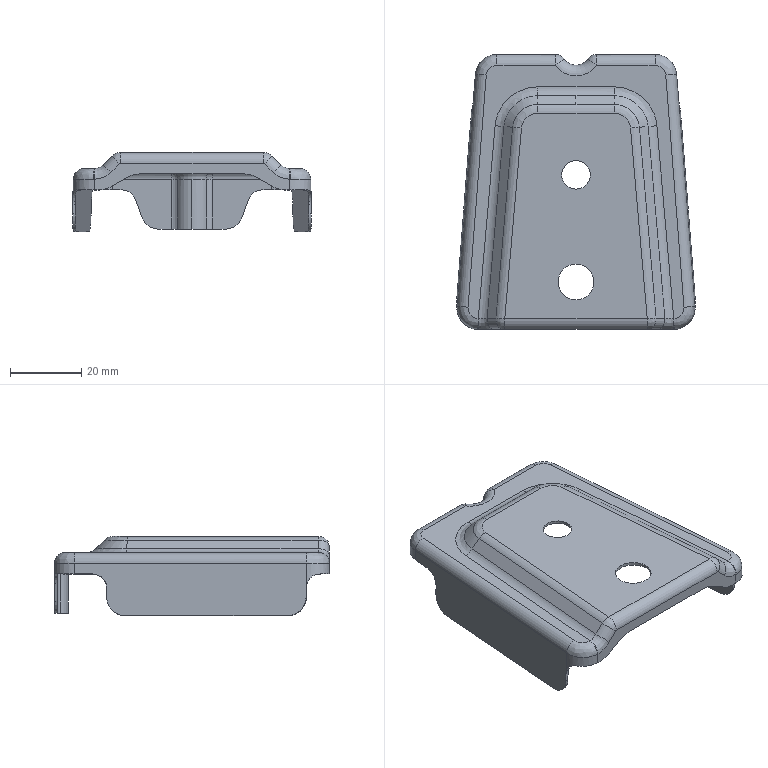Part | STEP file | FNA5401992 | 1 solid | 151 faces | box 66.933 x 77 x 22.144 mm | volume 6040 mm3 | spline 71 | cylinder 50 | plane 24 | sphere 4 | torus 2 | commonest cylinder face diameters 4.4 x9 6 x9 7 x6 12 x6 8 x4 10 x4